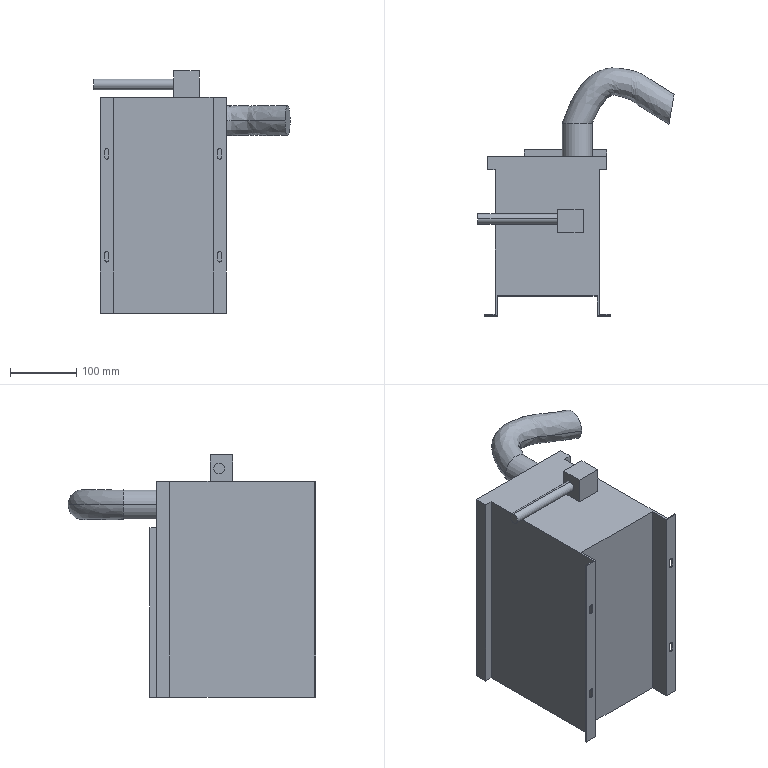Part | STEP file | Wrench controller | 1 solid | 59 faces | box 295.575 x 373.272 x 365 mm | volume 11651636 mm3 | plane 41 | cylinder 16 | spline 2 | commonest cylinder face diameters 6 x12 15.945 x2 45 x2